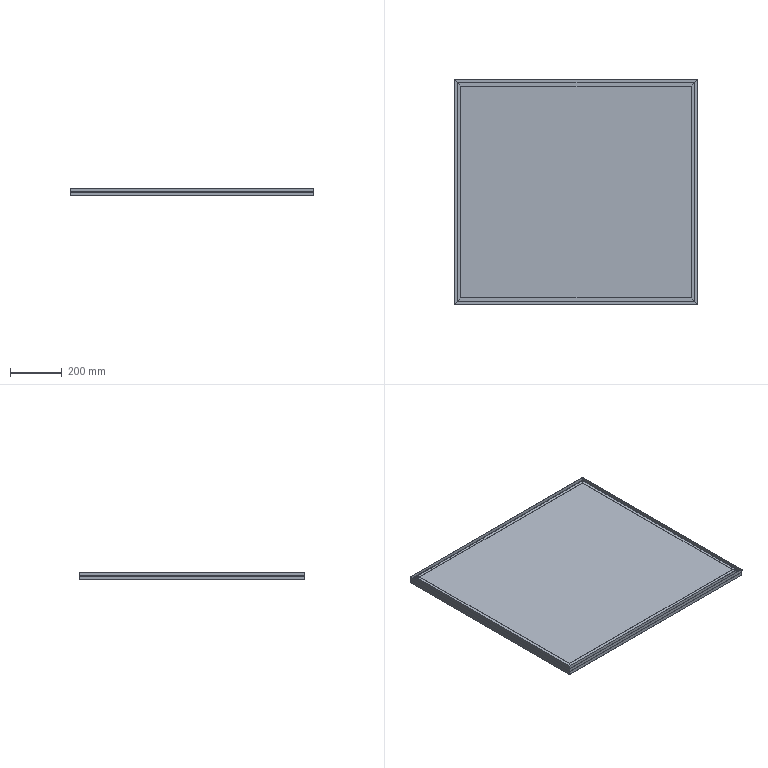Part | 5 solids | 78 faces | box 940 x 870 x 27 mm | volume 17299448 mm3 | plane 78